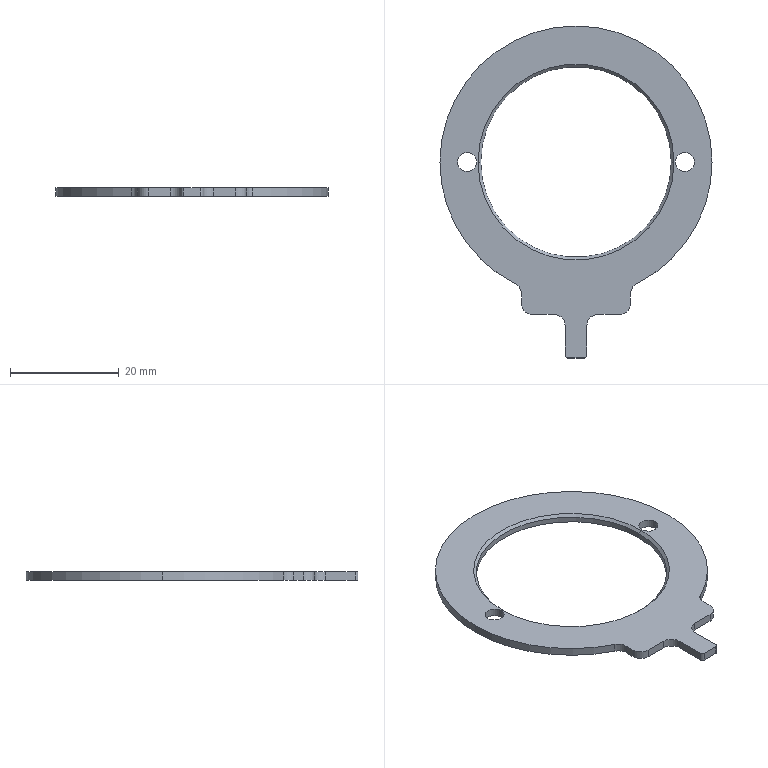Part | SolidWorks | features ICE 3, Fillet 2, Chamfer 1, Extrusion 1 | 1 solid | 28 faces | box 50 x 61 x 1.5 mm | volume 1619 mm3 | cylinder 17 | plane 9 | cone 2 | commonest cylinder face diameters 4 x6 3.5 x4 50 x3 1 x2 35 x2
STEP:
#1=CARTESIAN_POINT('',(-17.5,0.,1.));
#2=VERTEX_POINT('',#1);
#3=CARTESIAN_POINT('',(17.5,0.,1.));
#4=VERTEX_POINT('',#3);
#5=CARTESIAN_POINT('',(0.,0.,1.));
#6=DIRECTION('',(0.,0.,1.));
#7=DIRECTION('',(1.,0.,0.));
#8=AXIS2_PLACEMENT_3D('',#5,#6,#7);
#9=CIRCLE('',#8,17.5);
#10=EDGE_CURVE('',#2,#4,#9,.T.);
#11=ORIENTED_EDGE('',*,*,#10,.F.);
#12=CARTESIAN_POINT('',(-18.,0.,1.5));
#13=VERTEX_POINT('',#12);
#14=CARTESIAN_POINT('',(-17.5,0.,1.));
#15=DIRECTION('',(-0.7071,0.,0.7071));
#16=VECTOR('',#15,1000.);
#17=LINE('',#14,#16);
#18=EDGE_CURVE('',#2,#13,#17,.T.);
#19=ORIENTED_EDGE('',*,*,#18,.T.);
#20=CARTESIAN_POINT('',(18.,0.,1.5));
#21=VERTEX_POINT('',#20);
#22=CARTESIAN_POINT('',(0.,0.,1.5));
#23=DIRECTION('',(0.,0.,-1.));
#24=DIRECTION('',(1.,0.,0.));
#25=AXIS2_PLACEMENT_3D('',#22,#23,#24);
#26=CIRCLE('',#25,18.);
#27=EDGE_CURVE('',#21,#13,#26,.T.);
#28=ORIENTED_EDGE('',*,*,#27,.F.);
#29=CARTESIAN_POINT('',(17.5,0.,1.));
#30=DIRECTION('',(0.7071,0.,0.7071));
#31=VECTOR('',#30,1000.);
#32=LINE('',#29,#31);
#33=EDGE_CURVE('',#4,#21,#32,.T.);
#34=ORIENTED_EDGE('',*,*,#33,.F.);
#35=EDGE_LOOP('',(#11,#19,#28,#34));
#36=FACE_OUTER_BOUND('',#35,.T.);
#37=CARTESIAN_POINT('',(0.,0.,1.));
#38=DIRECTION('',(0.,0.,1.));
#39=DIRECTION('',(1.,0.,0.));
#40=AXIS2_PLACEMENT_3D('',#37,#38,#39);
#41=CONICAL_SURFACE('',#40,17.5,0.7854);
#42=ADVANCED_FACE('',(#36),#41,.F.);
#43=CARTESIAN_POINT('',(18.25,0.,0.));
#44=VERTEX_POINT('',#43);
#45=CARTESIAN_POINT('',(21.75,0.,0.));
#46=VERTEX_POINT('',#45);
#47=CARTESIAN_POINT('',(20.,0.,0.));
#48=DIRECTION('',(0.,0.,1.));
#49=DIRECTION('',(1.,0.,0.));
#50=AXIS2_PLACEMENT_3D('',#47,#48,#49);
#51=CIRCLE('',#50,1.75);
#52=EDGE_CURVE('',#44,#46,#51,.T.);
#53=ORIENTED_EDGE('',*,*,#52,.F.);
#54=CARTESIAN_POINT('',(18.25,0.,1.5));
#55=VERTEX_POINT('',#54);
#56=CARTESIAN_POINT('',(18.25,0.,-38.5));
#57=DIRECTION('',(0.,0.,1.));
#58=VECTOR('',#57,1000.);
#59=LINE('',#56,#58);
#60=EDGE_CURVE('',#44,#55,#59,.T.);
#61=ORIENTED_EDGE('',*,*,#60,.T.);
#62=CARTESIAN_POINT('',(21.75,0.,1.5));
#63=VERTEX_POINT('',#62);
#64=CARTESIAN_POINT('',(20.,0.,1.5));
#65=DIRECTION('',(0.,0.,1.));
#66=DIRECTION('',(1.,0.,0.));
#67=AXIS2_PLACEMENT_3D('',#64,#65,#66);
#68=CIRCLE('',#67,1.75);
#69=EDGE_CURVE('',#55,#63,#68,.T.);
#70=ORIENTED_EDGE('',*,*,#69,.T.);
#71=CARTESIAN_POINT('',(21.75,0.,-38.5));
#72=DIRECTION('',(0.,0.,1.));
#73=VECTOR('',#72,1000.);
#74=LINE('',#71,#73);
#75=EDGE_CURVE('',#46,#63,#74,.T.);
#76=ORIENTED_EDGE('',*,*,#75,.F.);
#77=EDGE_LOOP('',(#53,#61,#70,#76));
#78=FACE_OUTER_BOUND('',#77,.T.);
#79=CARTESIAN_POINT('',(20.,0.,-38.5));
#80=DIRECTION('',(0.,0.,1.));
#81=DIRECTION('',(1.,0.,0.));
#82=AXIS2_PLACEMENT_3D('',#79,#80,#81);
#83=CYLINDRICAL_SURFACE('',#82,1.75);
#84=ADVANCED_FACE('',(#78),#83,.F.);
#85=CARTESIAN_POINT('',(-21.75,0.,0.));
#86=VERTEX_POINT('',#85);
#87=CARTESIAN_POINT('',(-18.25,0.,0.));
#88=VERTEX_POINT('',#87);
#89=CARTESIAN_POINT('',(-20.,0.,0.));
#90=DIRECTION('',(0.,0.,1.));
#91=DIRECTION('',(1.,0.,0.));
#92=AXIS2_PLACEMENT_3D('',#89,#90,#91);
#93=CIRCLE('',#92,1.75);
#94=EDGE_CURVE('',#86,#88,#93,.T.);
#95=ORIENTED_EDGE('',*,*,#94,.F.);
#96=CARTESIAN_POINT('',(-21.75,0.,1.5));
#97=VERTEX_POINT('',#96);
#98=CARTESIAN_POINT('',(-21.75,0.,-38.5));
#99=DIRECTION('',(0.,0.,1.));
#100=VECTOR('',#99,1000.);
#101=LINE('',#98,#100);
#102=EDGE_CURVE('',#86,#97,#101,.T.);
#103=ORIENTED_EDGE('',*,*,#102,.T.);
#104=CARTESIAN_POINT('',(-18.25,0.,1.5));
#105=VERTEX_POINT('',#104);
#106=CARTESIAN_POINT('',(-20.,0.,1.5));
#107=DIRECTION('',(0.,0.,1.));
#108=DIRECTION('',(1.,0.,0.));
#109=AXIS2_PLACEMENT_3D('',#106,#107,#108);
#110=CIRCLE('',#109,1.75);
#111=EDGE_CURVE('',#97,#105,#110,.T.);
#112=ORIENTED_EDGE('',*,*,#111,.T.);
#113=CARTESIAN_POINT('',(-18.25,0.,-38.5));
#114=DIRECTION('',(0.,0.,1.));
#115=VECTOR('',#114,1000.);
#116=LINE('',#113,#115);
#117=EDGE_CURVE('',#88,#105,#116,.T.);
#118=ORIENTED_EDGE('',*,*,#117,.F.);
#119=EDGE_LOOP('',(#95,#103,#112,#118));
#120=FACE_OUTER_BOUND('',#119,.T.);
#121=CARTESIAN_POINT('',(-20.,0.,-38.5));
#122=DIRECTION('',(0.,0.,1.));
#123=DIRECTION('',(1.,0.,0.));
#124=AXIS2_PLACEMENT_3D('',#121,#122,#123);
#125=CYLINDRICAL_SURFACE('',#124,1.75);
#126=ADVANCED_FACE('',(#120),#125,.F.);
#127=ORIENTED_EDGE('',*,*,#10,.T.);
#128=CARTESIAN_POINT('',(17.5,0.,0.));
#129=VERTEX_POINT('',#128);
#130=CARTESIAN_POINT('',(17.5,0.,1.5));
#131=DIRECTION('',(0.,0.,-1.));
#132=VECTOR('',#131,1000.);
#133=LINE('',#130,#132);
#134=EDGE_CURVE('',#4,#129,#133,.T.);
#135=ORIENTED_EDGE('',*,*,#134,.T.);
#136=CARTESIAN_POINT('',(-17.5,0.,0.));
#137=VERTEX_POINT('',#136);
#138=CARTESIAN_POINT('',(0.,0.,0.));
#139=DIRECTION('',(0.,0.,1.));
#140=DIRECTION('',(1.,0.,0.));
#141=AXIS2_PLACEMENT_3D('',#138,#139,#140);
#142=CIRCLE('',#141,17.5);
#143=EDGE_CURVE('',#137,#129,#142,.T.);
#144=ORIENTED_EDGE('',*,*,#143,.F.);
#145=CARTESIAN_POINT('',(-17.5,0.,1.5));
#146=DIRECTION('',(0.,0.,-1.));
#147=VECTOR('',#146,1000.);
#148=LINE('',#145,#147);
#149=EDGE_CURVE('',#2,#137,#148,.T.);
#150=ORIENTED_EDGE('',*,*,#149,.F.);
#151=EDGE_LOOP('',(#127,#135,#144,#150));
#152=FACE_OUTER_BOUND('',#151,.T.);
#153=CARTESIAN_POINT('',(0.,0.,1.5));
#154=DIRECTION('',(0.,0.,-1.));
#155=DIRECTION('',(-1.,0.,0.));
#156=AXIS2_PLACEMENT_3D('',#153,#154,#155);
#157=CYLINDRICAL_SURFACE('',#156,17.5);
#158=ADVANCED_FACE('',(#152),#157,.F.);
#159=CARTESIAN_POINT('',(25.,0.,1.5));
#160=VERTEX_POINT('',#159);
#161=CARTESIAN_POINT('',(-25.,0.,1.5));
#162=VERTEX_POINT('',#161);
#163=CARTESIAN_POINT('',(0.,0.,1.5));
#164=DIRECTION('',(0.,0.,1.));
#165=DIRECTION('',(1.,0.,0.));
#166=AXIS2_PLACEMENT_3D('',#163,#164,#165);
#167=CIRCLE('',#166,25.);
#168=EDGE_CURVE('',#160,#162,#167,.T.);
#169=ORIENTED_EDGE('',*,*,#168,.F.);
#170=CARTESIAN_POINT('',(25.,0.,0.));
#171=VERTEX_POINT('',#170);
#172=CARTESIAN_POINT('',(25.,0.,1.5));
#173=DIRECTION('',(0.,0.,-1.));
#174=VECTOR('',#173,1000.);
#175=LINE('',#172,#174);
#176=EDGE_CURVE('',#160,#171,#175,.T.);
#177=ORIENTED_EDGE('',*,*,#176,.T.);
#178=CARTESIAN_POINT('',(-25.,0.,0.));
#179=VERTEX_POINT('',#178);
#180=CARTESIAN_POINT('',(0.,0.,0.));
#181=DIRECTION('',(0.,0.,1.));
#182=DIRECTION('',(1.,0.,0.));
#183=AXIS2_PLACEMENT_3D('',#180,#181,#182);
#184=CIRCLE('',#183,25.);
#185=EDGE_CURVE('',#171,#179,#184,.T.);
#186=ORIENTED_EDGE('',*,*,#185,.T.);
#187=CARTESIAN_POINT('',(-25.,0.,1.5));
#188=DIRECTION('',(0.,0.,-1.));
#189=VECTOR('',#188,1000.);
#190=LINE('',#187,#189);
#191=EDGE_CURVE('',#162,#179,#190,.T.);
#192=ORIENTED_EDGE('',*,*,#191,.F.);
#193=EDGE_LOOP('',(#169,#177,#186,#192));
#194=FACE_OUTER_BOUND('',#193,.T.);
#195=CARTESIAN_POINT('',(0.,0.,1.5));
#196=DIRECTION('',(0.,0.,-1.));
#197=DIRECTION('',(-1.,0.,0.));
#198=AXIS2_PLACEMENT_3D('',#195,#196,#197);
#199=CYLINDRICAL_SURFACE('',#198,25.);
#200=ADVANCED_FACE('',(#194),#199,.T.);
#201=CARTESIAN_POINT('',(-11.111,-22.395,1.5));
#202=VERTEX_POINT('',#201);
#203=CARTESIAN_POINT('',(0.,0.,1.5));
#204=DIRECTION('',(0.,0.,1.));
#205=DIRECTION('',(1.,0.,0.));
#206=AXIS2_PLACEMENT_3D('',#203,#204,#205);
#207=CIRCLE('',#206,25.);
#208=EDGE_CURVE('',#162,#202,#207,.T.);
#209=ORIENTED_EDGE('',*,*,#208,.F.);
#210=ORIENTED_EDGE('',*,*,#191,.T.);
#211=CARTESIAN_POINT('',(-11.111,-22.395,0.));
#212=VERTEX_POINT('',#211);
#213=CARTESIAN_POINT('',(0.,0.,0.));
#214=DIRECTION('',(0.,0.,1.));
#215=DIRECTION('',(1.,0.,0.));
#216=AXIS2_PLACEMENT_3D('',#213,#214,#215);
#217=CIRCLE('',#216,25.);
#218=EDGE_CURVE('',#179,#212,#217,.T.);
#219=ORIENTED_EDGE('',*,*,#218,.T.);
#220=CARTESIAN_POINT('',(-11.111,-22.395,1.5));
#221=DIRECTION('',(0.,0.,1.));
#222=VECTOR('',#221,1000.);
#223=LINE('',#220,#222);
#224=EDGE_CURVE('',#212,#202,#223,.T.);
#225=ORIENTED_EDGE('',*,*,#224,.T.);
#226=EDGE_LOOP('',(#209,#210,#219,#225));
#227=FACE_OUTER_BOUND('',#226,.T.);
#228=CARTESIAN_POINT('',(0.,0.,1.5));
#229=DIRECTION('',(0.,0.,-1.));
#230=DIRECTION('',(-1.,0.,0.));
#231=AXIS2_PLACEMENT_3D('',#228,#229,#230);
#232=CYLINDRICAL_SURFACE('',#231,25.);
#233=ADVANCED_FACE('',(#227),#232,.T.);
#234=ORIENTED_EDGE('',*,*,#27,.T.);
#235=CARTESIAN_POINT('',(0.,0.,1.5));
#236=DIRECTION('',(0.,0.,-1.));
#237=DIRECTION('',(1.,0.,0.));
#238=AXIS2_PLACEMENT_3D('',#235,#236,#237);
#239=CIRCLE('',#238,18.);
#240=EDGE_CURVE('',#13,#21,#239,.T.);
#241=ORIENTED_EDGE('',*,*,#240,.T.);
#242=EDGE_LOOP('',(#234,#241));
#243=FACE_BOUND('',#242,.T.);
#244=CARTESIAN_POINT('',(20.,0.,1.5));
#245=DIRECTION('',(0.,0.,1.));
#246=DIRECTION('',(1.,0.,0.));
#247=AXIS2_PLACEMENT_3D('',#244,#245,#246);
#248=CIRCLE('',#247,1.75);
#249=EDGE_CURVE('',#63,#55,#248,.T.);
#250=ORIENTED_EDGE('',*,*,#249,.F.);
#251=ORIENTED_EDGE('',*,*,#69,.F.);
#252=EDGE_LOOP('',(#250,#251));
#253=FACE_BOUND('',#252,.T.);
#254=CARTESIAN_POINT('',(-20.,0.,1.5));
#255=DIRECTION('',(0.,0.,1.));
#256=DIRECTION('',(1.,0.,0.));
#257=AXIS2_PLACEMENT_3D('',#254,#255,#256);
#258=CIRCLE('',#257,1.75);
#259=EDGE_CURVE('',#105,#97,#258,.T.);
#260=ORIENTED_EDGE('',*,*,#259,.F.);
#261=ORIENTED_EDGE('',*,*,#111,.F.);
#262=EDGE_LOOP('',(#260,#261));
#263=FACE_BOUND('',#262,.T.);
#264=CARTESIAN_POINT('',(-1.5,-36.,1.5));
#265=VERTEX_POINT('',#264);
#266=CARTESIAN_POINT('',(1.5,-36.,1.5));
#267=VERTEX_POINT('',#266);
#268=CARTESIAN_POINT('',(-10.,-36.,1.5));
#269=DIRECTION('',(1.,0.,0.));
#270=VECTOR('',#269,1000.);
#271=LINE('',#268,#270);
#272=EDGE_CURVE('',#265,#267,#271,.T.);
#273=ORIENTED_EDGE('',*,*,#272,.T.);
#274=CARTESIAN_POINT('',(2.,-35.5,1.5));
#275=VERTEX_POINT('',#274);
#276=CARTESIAN_POINT('',(1.5,-35.5,1.5));
#277=DIRECTION('',(0.,0.,1.));
#278=DIRECTION('',(1.,0.,0.));
#279=AXIS2_PLACEMENT_3D('',#276,#277,#278);
#280=CIRCLE('',#279,0.5);
#281=EDGE_CURVE('',#267,#275,#280,.T.);
#282=ORIENTED_EDGE('',*,*,#281,.T.);
#283=CARTESIAN_POINT('',(2.,-30.,1.5));
#284=VERTEX_POINT('',#283);
#285=CARTESIAN_POINT('',(2.,-36.,1.5));
#286=DIRECTION('',(0.,-1.,0.));
#287=VECTOR('',#286,1000.);
#288=LINE('',#285,#287);
#289=EDGE_CURVE('',#284,#275,#288,.T.);
#290=ORIENTED_EDGE('',*,*,#289,.F.);
#291=CARTESIAN_POINT('',(4.,-28.,1.5));
#292=VERTEX_POINT('',#291);
#293=CARTESIAN_POINT('',(4.,-30.,1.5));
#294=DIRECTION('',(0.,0.,-1.));
#295=DIRECTION('',(1.,0.,0.));
#296=AXIS2_PLACEMENT_3D('',#293,#294,#295);
#297=CIRCLE('',#296,2.);
#298=EDGE_CURVE('',#284,#292,#297,.T.);
#299=ORIENTED_EDGE('',*,*,#298,.T.);
#300=CARTESIAN_POINT('',(8.,-28.,1.5));
#301=VERTEX_POINT('',#300);
#302=CARTESIAN_POINT('',(10.,-28.,1.5));
#303=DIRECTION('',(-1.,0.,0.));
#304=VECTOR('',#303,1000.);
#305=LINE('',#302,#304);
#306=EDGE_CURVE('',#301,#292,#305,.T.);
#307=ORIENTED_EDGE('',*,*,#306,.F.);
#308=CARTESIAN_POINT('',(10.,-26.,1.5));
#309=VERTEX_POINT('',#308);
#310=CARTESIAN_POINT('',(8.,-26.,1.5));
#311=DIRECTION('',(0.,0.,1.));
#312=DIRECTION('',(1.,0.,0.));
#313=AXIS2_PLACEMENT_3D('',#310,#311,#312);
#314=CIRCLE('',#313,2.);
#315=EDGE_CURVE('',#301,#309,#314,.T.);
#316=ORIENTED_EDGE('',*,*,#315,.T.);
#317=CARTESIAN_POINT('',(10.,-24.187,1.5));
#318=VERTEX_POINT('',#317);
#319=CARTESIAN_POINT('',(10.,-21.,1.5));
#320=DIRECTION('',(0.,1.,0.));
#321=VECTOR('',#320,1000.);
#322=LINE('',#319,#321);
#323=EDGE_CURVE('',#309,#318,#322,.T.);
#324=ORIENTED_EDGE('',*,*,#323,.T.);
#325=CARTESIAN_POINT('',(11.111,-22.395,1.5));
#326=VERTEX_POINT('',#325);
#327=CARTESIAN_POINT('',(12.,-24.187,1.5));
#328=DIRECTION('',(0.,0.,-1.));
#329=DIRECTION('',(1.,0.,0.));
#330=AXIS2_PLACEMENT_3D('',#327,#328,#329);
#331=CIRCLE('',#330,2.);
#332=EDGE_CURVE('',#318,#326,#331,.T.);
#333=ORIENTED_EDGE('',*,*,#332,.T.);
#334=CARTESIAN_POINT('',(0.,0.,1.5));
#335=DIRECTION('',(0.,0.,1.));
#336=DIRECTION('',(1.,0.,0.));
#337=AXIS2_PLACEMENT_3D('',#334,#335,#336);
#338=CIRCLE('',#337,25.);
#339=EDGE_CURVE('',#326,#160,#338,.T.);
#340=ORIENTED_EDGE('',*,*,#339,.T.);
#341=ORIENTED_EDGE('',*,*,#168,.T.);
#342=ORIENTED_EDGE('',*,*,#208,.T.);
#343=CARTESIAN_POINT('',(-10.,-24.187,1.5));
#344=VERTEX_POINT('',#343);
#345=CARTESIAN_POINT('',(-12.,-24.187,1.5));
#346=DIRECTION('',(0.,0.,-1.));
#347=DIRECTION('',(1.,0.,0.));
#348=AXIS2_PLACEMENT_3D('',#345,#346,#347);
#349=CIRCLE('',#348,2.);
#350=EDGE_CURVE('',#202,#344,#349,.T.);
#351=ORIENTED_EDGE('',*,*,#350,.T.);
#352=CARTESIAN_POINT('',(-10.,-26.,1.5));
#353=VERTEX_POINT('',#352);
#354=CARTESIAN_POINT('',(-10.,-21.,1.5));
#355=DIRECTION('',(0.,-1.,0.));
#356=VECTOR('',#355,1000.);
#357=LINE('',#354,#356);
#358=EDGE_CURVE('',#344,#353,#357,.T.);
#359=ORIENTED_EDGE('',*,*,#358,.T.);
#360=CARTESIAN_POINT('',(-8.,-28.,1.5));
#361=VERTEX_POINT('',#360);
#362=CARTESIAN_POINT('',(-8.,-26.,1.5));
#363=DIRECTION('',(0.,0.,1.));
#364=DIRECTION('',(1.,0.,0.));
#365=AXIS2_PLACEMENT_3D('',#362,#363,#364);
#366=CIRCLE('',#365,2.);
#367=EDGE_CURVE('',#353,#361,#366,.T.);
#368=ORIENTED_EDGE('',*,*,#367,.T.);
#369=CARTESIAN_POINT('',(-4.,-28.,1.5));
#370=VERTEX_POINT('',#369);
#371=CARTESIAN_POINT('',(-10.,-28.,1.5));
#372=DIRECTION('',(-1.,0.,0.));
#373=VECTOR('',#372,1000.);
#374=LINE('',#371,#373);
#375=EDGE_CURVE('',#370,#361,#374,.T.);
#376=ORIENTED_EDGE('',*,*,#375,.F.);
#377=CARTESIAN_POINT('',(-2.,-30.,1.5));
#378=VERTEX_POINT('',#377);
#379=CARTESIAN_POINT('',(-4.,-30.,1.5));
#380=DIRECTION('',(0.,0.,-1.));
#381=DIRECTION('',(1.,0.,0.));
#382=AXIS2_PLACEMENT_3D('',#379,#380,#381);
#383=CIRCLE('',#382,2.);
#384=EDGE_CURVE('',#370,#378,#383,.T.);
#385=ORIENTED_EDGE('',*,*,#384,.T.);
#386=CARTESIAN_POINT('',(-2.,-35.5,1.5));
#387=VERTEX_POINT('',#386);
#388=CARTESIAN_POINT('',(-2.,-36.,1.5));
#389=DIRECTION('',(0.,1.,0.));
#390=VECTOR('',#389,1000.);
#391=LINE('',#388,#390);
#392=EDGE_CURVE('',#387,#378,#391,.T.);
#393=ORIENTED_EDGE('',*,*,#392,.F.);
#394=CARTESIAN_POINT('',(-1.5,-35.5,1.5));
#395=DIRECTION('',(0.,0.,1.));
#396=DIRECTION('',(1.,0.,0.));
#397=AXIS2_PLACEMENT_3D('',#394,#395,#396);
#398=CIRCLE('',#397,0.5);
#399=EDGE_CURVE('',#387,#265,#398,.T.);
#400=ORIENTED_EDGE('',*,*,#399,.T.);
#401=EDGE_LOOP('',(#273,#282,#290,#299,#307,#316,#324,#333,#340,#341,#342,#351,#359,#368,#376,#385,#393,#400));
#402=FACE_OUTER_BOUND('',#401,.T.);
#403=CARTESIAN_POINT('',(0.,0.,1.5));
#404=DIRECTION('',(0.,0.,1.));
#405=DIRECTION('',(1.,0.,0.));
#406=AXIS2_PLACEMENT_3D('',#403,#404,#405);
#407=PLANE('',#406);
#408=ADVANCED_FACE('',(#243,#253,#263,#402),#407,.T.);
#409=CARTESIAN_POINT('',(20.,0.,0.));
#410=DIRECTION('',(0.,0.,1.));
#411=DIRECTION('',(1.,0.,0.));
#412=AXIS2_PLACEMENT_3D('',#409,#410,#411);
#413=CIRCLE('',#412,1.75);
#414=EDGE_CURVE('',#46,#44,#413,.T.);
#415=ORIENTED_EDGE('',*,*,#414,.T.);
#416=ORIENTED_EDGE('',*,*,#52,.T.);
#417=EDGE_LOOP('',(#415,#416));
#418=FACE_BOUND('',#417,.T.);
#419=CARTESIAN_POINT('',(-20.,0.,0.));
#420=DIRECTION('',(0.,0.,1.));
#421=DIRECTION('',(1.,0.,0.));
#422=AXIS2_PLACEMENT_3D('',#419,#420,#421);
#423=CIRCLE('',#422,1.75);
#424=EDGE_CURVE('',#88,#86,#423,.T.);
#425=ORIENTED_EDGE('',*,*,#424,.T.);
#426=ORIENTED_EDGE('',*,*,#94,.T.);
#427=EDGE_LOOP('',(#425,#426));
#428=FACE_BOUND('',#427,.T.);
#429=CARTESIAN_POINT('',(2.,-30.,0.));
#430=VERTEX_POINT('',#429);
#431=CARTESIAN_POINT('',(2.,-35.5,0.));
#432=VERTEX_POINT('',#431);
#433=CARTESIAN_POINT('',(2.,0.,0.));
#434=DIRECTION('',(0.,-1.,0.));
#435=VECTOR('',#434,1000.);
#436=LINE('',#433,#435);
#437=EDGE_CURVE('',#430,#432,#436,.T.);
#438=ORIENTED_EDGE('',*,*,#437,.T.);
#439=CARTESIAN_POINT('',(1.5,-36.,0.));
#440=VERTEX_POINT('',#439);
#441=CARTESIAN_POINT('',(1.5,-35.5,0.));
#442=DIRECTION('',(0.,0.,-1.));
#443=DIRECTION('',(1.,0.,0.));
#444=AXIS2_PLACEMENT_3D('',#441,#442,#443);
#445=CIRCLE('',#444,0.5);
#446=EDGE_CURVE('',#432,#440,#445,.T.);
#447=ORIENTED_EDGE('',*,*,#446,.T.);
#448=CARTESIAN_POINT('',(-1.5,-36.,0.));
#449=VERTEX_POINT('',#448);
#450=CARTESIAN_POINT('',(-10.,-36.,0.));
#451=DIRECTION('',(-1.,0.,0.));
#452=VECTOR('',#451,1000.);
#453=LINE('',#450,#452);
#454=EDGE_CURVE('',#440,#449,#453,.T.);
#455=ORIENTED_EDGE('',*,*,#454,.T.);
#456=CARTESIAN_POINT('',(-2.,-35.5,0.));
#457=VERTEX_POINT('',#456);
#458=CARTESIAN_POINT('',(-1.5,-35.5,0.));
#459=DIRECTION('',(0.,0.,-1.));
#460=DIRECTION('',(1.,0.,0.));
#461=AXIS2_PLACEMENT_3D('',#458,#459,#460);
#462=CIRCLE('',#461,0.5);
#463=EDGE_CURVE('',#449,#457,#462,.T.);
#464=ORIENTED_EDGE('',*,*,#463,.T.);
#465=CARTESIAN_POINT('',(-2.,-30.,0.));
#466=VERTEX_POINT('',#465);
#467=CARTESIAN_POINT('',(-2.,0.,0.));
#468=DIRECTION('',(0.,1.,0.));
#469=VECTOR('',#468,1000.);
#470=LINE('',#467,#469);
#471=EDGE_CURVE('',#457,#466,#470,.T.);
#472=ORIENTED_EDGE('',*,*,#471,.T.);
#473=CARTESIAN_POINT('',(-4.,-28.,0.));
#474=VERTEX_POINT('',#473);
#475=CARTESIAN_POINT('',(-4.,-30.,0.));
#476=DIRECTION('',(0.,0.,1.));
#477=DIRECTION('',(1.,0.,0.));
#478=AXIS2_PLACEMENT_3D('',#475,#476,#477);
#479=CIRCLE('',#478,2.);
#480=EDGE_CURVE('',#466,#474,#479,.T.);
#481=ORIENTED_EDGE('',*,*,#480,.T.);
#482=CARTESIAN_POINT('',(-8.,-28.,0.));
#483=VERTEX_POINT('',#482);
#484=CARTESIAN_POINT('',(0.,-28.,0.));
#485=DIRECTION('',(-1.,0.,0.));
#486=VECTOR('',#485,1000.);
#487=LINE('',#484,#486);
#488=EDGE_CURVE('',#474,#483,#487,.T.);
#489=ORIENTED_EDGE('',*,*,#488,.T.);
#490=CARTESIAN_POINT('',(-10.,-26.,0.));
#491=VERTEX_POINT('',#490);
#492=CARTESIAN_POINT('',(-8.,-26.,0.));
#493=DIRECTION('',(0.,0.,-1.));
#494=DIRECTION('',(1.,0.,0.));
#495=AXIS2_PLACEMENT_3D('',#492,#493,#494);
#496=CIRCLE('',#495,2.);
#497=EDGE_CURVE('',#483,#491,#496,.T.);
#498=ORIENTED_EDGE('',*,*,#497,.T.);
#499=CARTESIAN_POINT('',(-10.,-24.187,0.));
#500=VERTEX_POINT('',#499);
#501=CARTESIAN_POINT('',(-10.,-21.,0.));
#502=DIRECTION('',(0.,1.,0.));
#503=VECTOR('',#502,1000.);
#504=LINE('',#501,#503);
#505=EDGE_CURVE('',#491,#500,#504,.T.);
#506=ORIENTED_EDGE('',*,*,#505,.T.);
#507=CARTESIAN_POINT('',(-12.,-24.187,0.));
#508=DIRECTION('',(0.,0.,1.));
#509=DIRECTION('',(1.,0.,0.));
#510=AXIS2_PLACEMENT_3D('',#507,#508,#509);
#511=CIRCLE('',#510,2.);
#512=EDGE_CURVE('',#500,#212,#511,.T.);
#513=ORIENTED_EDGE('',*,*,#512,.T.);
#514=ORIENTED_EDGE('',*,*,#218,.F.);
#515=ORIENTED_EDGE('',*,*,#185,.F.);
#516=CARTESIAN_POINT('',(11.111,-22.395,0.));
#517=VERTEX_POINT('',#516);
#518=CARTESIAN_POINT('',(0.,0.,0.));
#519=DIRECTION('',(0.,0.,1.));
#520=DIRECTION('',(1.,0.,0.));
#521=AXIS2_PLACEMENT_3D('',#518,#519,#520);
#522=CIRCLE('',#521,25.);
#523=EDGE_CURVE('',#517,#171,#522,.T.);
#524=ORIENTED_EDGE('',*,*,#523,.F.);
#525=CARTESIAN_POINT('',(10.,-24.187,0.));
#526=VERTEX_POINT('',#525);
#527=CARTESIAN_POINT('',(12.,-24.187,0.));
#528=DIRECTION('',(0.,0.,1.));
#529=DIRECTION('',(1.,0.,0.));
#530=AXIS2_PLACEMENT_3D('',#527,#528,#529);
#531=CIRCLE('',#530,2.);
#532=EDGE_CURVE('',#517,#526,#531,.T.);
#533=ORIENTED_EDGE('',*,*,#532,.T.);
#534=CARTESIAN_POINT('',(10.,-26.,0.));
#535=VERTEX_POINT('',#534);
#536=CARTESIAN_POINT('',(10.,-21.,0.));
#537=DIRECTION('',(0.,-1.,0.));
#538=VECTOR('',#537,1000.);
#539=LINE('',#536,#538);
#540=EDGE_CURVE('',#526,#535,#539,.T.);
#541=ORIENTED_EDGE('',*,*,#540,.T.);
#542=CARTESIAN_POINT('',(8.,-28.,0.));
#543=VERTEX_POINT('',#542);
#544=CARTESIAN_POINT('',(8.,-26.,0.));
#545=DIRECTION('',(0.,0.,-1.));
#546=DIRECTION('',(1.,0.,0.));
#547=AXIS2_PLACEMENT_3D('',#544,#545,#546);
#548=CIRCLE('',#547,2.);
#549=EDGE_CURVE('',#535,#543,#548,.T.);
#550=ORIENTED_EDGE('',*,*,#549,.T.);
#551=CARTESIAN_POINT('',(4.,-28.,0.));
#552=VERTEX_POINT('',#551);
#553=CARTESIAN_POINT('',(0.,-28.,0.));
#554=DIRECTION('',(-1.,0.,0.));
#555=VECTOR('',#554,1000.);
#556=LINE('',#553,#555);
#557=EDGE_CURVE('',#543,#552,#556,.T.);
#558=ORIENTED_EDGE('',*,*,#557,.T.);
#559=CARTESIAN_POINT('',(4.,-30.,0.));
#560=DIRECTION('',(0.,0.,1.));
#561=DIRECTION('',(1.,0.,0.));
#562=AXIS2_PLACEMENT_3D('',#559,#560,#561);
#563=CIRCLE('',#562,2.);
#564=EDGE_CURVE('',#552,#430,#563,.T.);
#565=ORIENTED_EDGE('',*,*,#564,.T.);
#566=EDGE_LOOP('',(#438,#447,#455,#464,#472,#481,#489,#498,#506,#513,#514,#515,#524,#533,#541,#550,#558,#565));
#567=FACE_OUTER_BOUND('',#566,.T.);
#568=ORIENTED_EDGE('',*,*,#143,.T.);
#569=CARTESIAN_POINT('',(0.,0.,0.));
#570=DIRECTION('',(0.,0.,1.));
#571=DIRECTION('',(1.,0.,0.));
#572=AXIS2_PLACEMENT_3D('',#569,#570,#571);
#573=CIRCLE('',#572,17.5);
#574=EDGE_CURVE('',#129,#137,#573,.T.);
#575=ORIENTED_EDGE('',*,*,#574,.T.);
#576=EDGE_LOOP('',(#568,#575));
#577=FACE_BOUND('',#576,.T.);
#578=CARTESIAN_POINT('',(0.,0.,0.));
#579=DIRECTION('',(0.,0.,1.));
#580=DIRECTION('',(1.,0.,0.));
#581=AXIS2_PLACEMENT_3D('',#578,#579,#580);
#582=PLANE('',#581);
#583=ADVANCED_FACE('',(#418,#428,#567,#577),#582,.F.);
#584=ORIENTED_EDGE('',*,*,#176,.F.);
#585=ORIENTED_EDGE('',*,*,#339,.F.);
#586=CARTESIAN_POINT('',(11.111,-22.395,1.5));
#587=DIRECTION('',(0.,0.,-1.));
#588=VECTOR('',#587,1000.);
#589=LINE('',#586,#588);
#590=EDGE_CURVE('',#326,#517,#589,.T.);
#591=ORIENTED_EDGE('',*,*,#590,.T.);
#592=ORIENTED_EDGE('',*,*,#523,.T.);
#593=EDGE_LOOP('',(#584,#585,#591,#592));
#594=FACE_OUTER_BOUND('',#593,.T.);
#595=CARTESIAN_POINT('',(0.,0.,1.5));
#596=DIRECTION('',(0.,0.,-1.));
#597=DIRECTION('',(-1.,0.,0.));
#598=AXIS2_PLACEMENT_3D('',#595,#596,#597);
#599=CYLINDRICAL_SURFACE('',#598,25.);
#600=ADVANCED_FACE('',(#594),#599,.T.);
#601=ORIENTED_EDGE('',*,*,#134,.F.);
#602=CARTESIAN_POINT('',(0.,0.,1.));
#603=DIRECTION('',(0.,0.,1.));
#604=DIRECTION('',(1.,0.,0.));
#605=AXIS2_PLACEMENT_3D('',#602,#603,#604);
#606=CIRCLE('',#605,17.5);
#607=EDGE_CURVE('',#4,#2,#606,.T.);
#608=ORIENTED_EDGE('',*,*,#607,.T.);
#609=ORIENTED_EDGE('',*,*,#149,.T.);
#610=ORIENTED_EDGE('',*,*,#574,.F.);
#611=EDGE_LOOP('',(#601,#608,#609,#610));
#612=FACE_OUTER_BOUND('',#611,.T.);
#613=CARTESIAN_POINT('',(0.,0.,1.5));
#614=DIRECTION('',(0.,0.,-1.));
#615=DIRECTION('',(-1.,0.,0.));
#616=AXIS2_PLACEMENT_3D('',#613,#614,#615);
#617=CYLINDRICAL_SURFACE('',#616,17.5);
#618=ADVANCED_FACE('',(#612),#617,.F.);
#619=ORIENTED_EDGE('',*,*,#505,.F.);
#620=CARTESIAN_POINT('',(-10.,-26.,1.5));
#621=DIRECTION('',(0.,0.,1.));
#622=VECTOR('',#621,1000.);
#623=LINE('',#620,#622);
#624=EDGE_CURVE('',#491,#353,#623,.T.);
#625=ORIENTED_EDGE('',*,*,#624,.T.);
#626=ORIENTED_EDGE('',*,*,#358,.F.);
#627=CARTESIAN_POINT('',(-10.,-24.187,-25.));
#628=DIRECTION('',(0.,0.,-1.));
#629=VECTOR('',#628,1000.);
#630=LINE('',#627,#629);
#631=EDGE_CURVE('',#344,#500,#630,.T.);
#632=ORIENTED_EDGE('',*,*,#631,.T.);
#633=EDGE_LOOP('',(#619,#625,#626,#632));
#634=FACE_OUTER_BOUND('',#633,.T.);
#635=CARTESIAN_POINT('',(-10.,-21.,-25.));
#636=DIRECTION('',(-1.,0.,0.));
#637=DIRECTION('',(0.,-1.,0.));
#638=AXIS2_PLACEMENT_3D('',#635,#636,#637);
#639=PLANE('',#638);
#640=ADVANCED_FACE('',(#634),#639,.T.);
#641=ORIENTED_EDGE('',*,*,#323,.F.);
#642=CARTESIAN_POINT('',(10.,-26.,0.));
#643=DIRECTION('',(0.,0.,-1.));
#644=VECTOR('',#643,1000.);
#645=LINE('',#642,#644);
#646=EDGE_CURVE('',#309,#535,#645,.T.);
#647=ORIENTED_EDGE('',*,*,#646,.T.);
#648=ORIENTED_EDGE('',*,*,#540,.F.);
#649=CARTESIAN_POINT('',(10.,-24.187,-25.));
#650=DIRECTION('',(0.,0.,1.));
#651=VECTOR('',#650,1000.);
#652=LINE('',#649,#651);
#653=EDGE_CURVE('',#526,#318,#652,.T.);
#654=ORIENTED_EDGE('',*,*,#653,.T.);
#655=EDGE_LOOP('',(#641,#647,#648,#654));
#656=FACE_OUTER_BOUND('',#655,.T.);
#657=CARTESIAN_POINT('',(10.,-21.,-25.));
#658=DIRECTION('',(1.,0.,0.));
#659=DIRECTION('',(0.,1.,0.));
#660=AXIS2_PLACEMENT_3D('',#657,#658,#659);
#661=PLANE('',#660);
#662=ADVANCED_FACE('',(#656),#661,.T.);
#663=ORIENTED_EDGE('',*,*,#454,.F.);
#664=CARTESIAN_POINT('',(1.5,-36.,1.5));
#665=DIRECTION('',(0.,0.,1.));
#666=VECTOR('',#665,1000.);
#667=LINE('',#664,#666);
#668=EDGE_CURVE('',#440,#267,#667,.T.);
#669=ORIENTED_EDGE('',*,*,#668,.T.);
#670=ORIENTED_EDGE('',*,*,#272,.F.);
#671=CARTESIAN_POINT('',(-1.5,-36.,0.));
#672=DIRECTION('',(0.,0.,-1.));
#673=VECTOR('',#672,1000.);
#674=LINE('',#671,#673);
#675=EDGE_CURVE('',#265,#449,#674,.T.);
#676=ORIENTED_EDGE('',*,*,#675,.T.);
#677=EDGE_LOOP('',(#663,#669,#670,#676));
#678=FACE_OUTER_BOUND('',#677,.T.);
#679=CARTESIAN_POINT('',(-10.,-36.,-25.));
#680=DIRECTION('',(0.,-1.,0.));
#681=DIRECTION('',(0.,0.,-1.));
#682=AXIS2_PLACEMENT_3D('',#679,#680,#681);
#683=PLANE('',#682);
#684=ADVANCED_FACE('',(#678),#683,.T.);
#685=ORIENTED_EDGE('',*,*,#375,.T.);
#686=CARTESIAN_POINT('',(-8.,-28.,0.));
#687=DIRECTION('',(0.,0.,-1.));
#688=VECTOR('',#687,1000.);
#689=LINE('',#686,#688);
#690=EDGE_CURVE('',#361,#483,#689,.T.);
#691=ORIENTED_EDGE('',*,*,#690,.T.);
#692=ORIENTED_EDGE('',*,*,#488,.F.);
#693=CARTESIAN_POINT('',(-4.,-28.,1.5));
#694=DIRECTION('',(0.,0.,1.));
#695=VECTOR('',#694,1000.);
#696=LINE('',#693,#695);
#697=EDGE_CURVE('',#474,#370,#696,.T.);
#698=ORIENTED_EDGE('',*,*,#697,.T.);
#699=EDGE_LOOP('',(#685,#691,#692,#698));
#700=FACE_OUTER_BOUND('',#699,.T.);
#701=CARTESIAN_POINT('',(-10.,-28.,-18.5));
#702=DIRECTION('',(0.,1.,0.));
#703=DIRECTION('',(0.,0.,1.));
#704=AXIS2_PLACEMENT_3D('',#701,#702,#703);
#705=PLANE('',#704);
#706=ADVANCED_FACE('',(#700),#705,.F.);
#707=ORIENTED_EDGE('',*,*,#471,.F.);
#708=CARTESIAN_POINT('',(-2.,-35.5,1.5));
#709=DIRECTION('',(0.,0.,1.));
#710=VECTOR('',#709,1000.);
#711=LINE('',#708,#710);
#712=EDGE_CURVE('',#457,#387,#711,.T.);
#713=ORIENTED_EDGE('',*,*,#712,.T.);
#714=ORIENTED_EDGE('',*,*,#392,.T.);
#715=CARTESIAN_POINT('',(-2.,-30.,0.));
#716=DIRECTION('',(0.,0.,-1.));
#717=VECTOR('',#716,1000.);
#718=LINE('',#715,#717);
#719=EDGE_CURVE('',#378,#466,#718,.T.);
#720=ORIENTED_EDGE('',*,*,#719,.T.);
#721=EDGE_LOOP('',(#707,#713,#714,#720));
#722=FACE_OUTER_BOUND('',#721,.T.);
#723=CARTESIAN_POINT('',(-2.,-36.,-18.5));
#724=DIRECTION('',(1.,0.,0.));
#725=DIRECTION('',(0.,0.,-1.));
#726=AXIS2_PLACEMENT_3D('',#723,#724,#725);
#727=PLANE('',#726);
#728=ADVANCED_FACE('',(#722),#727,.F.);
#729=ORIENTED_EDGE('',*,*,#557,.F.);
#730=CARTESIAN_POINT('',(8.,-28.,1.5));
#731=DIRECTION('',(0.,0.,1.));
#732=VECTOR('',#731,1000.);
#733=LINE('',#730,#732);
#734=EDGE_CURVE('',#543,#301,#733,.T.);
#735=ORIENTED_EDGE('',*,*,#734,.T.);
#736=ORIENTED_EDGE('',*,*,#306,.T.);
#737=CARTESIAN_POINT('',(4.,-28.,0.));
#738=DIRECTION('',(0.,0.,-1.));
#739=VECTOR('',#738,1000.);
#740=LINE('',#737,#739);
#741=EDGE_CURVE('',#292,#552,#740,.T.);
#742=ORIENTED_EDGE('',*,*,#741,.T.);
#743=EDGE_LOOP('',(#729,#735,#736,#742));
#744=FACE_OUTER_BOUND('',#743,.T.);
#745=CARTESIAN_POINT('',(10.,-28.,-18.5));
#746=DIRECTION('',(0.,1.,0.));
#747=DIRECTION('',(0.,0.,1.));
#748=AXIS2_PLACEMENT_3D('',#745,#746,#747);
#749=PLANE('',#748);
#750=ADVANCED_FACE('',(#744),#749,.F.);
#751=ORIENTED_EDGE('',*,*,#289,.T.);
#752=CARTESIAN_POINT('',(2.,-35.5,0.));
#753=DIRECTION('',(0.,0.,-1.));
#754=VECTOR('',#753,1000.);
#755=LINE('',#752,#754);
#756=EDGE_CURVE('',#275,#432,#755,.T.);
#757=ORIENTED_EDGE('',*,*,#756,.T.);
#758=ORIENTED_EDGE('',*,*,#437,.F.);
#759=CARTESIAN_POINT('',(2.,-30.,1.5));
#760=DIRECTION('',(0.,0.,1.));
#761=VECTOR('',#760,1000.);
#762=LINE('',#759,#761);
#763=EDGE_CURVE('',#430,#284,#762,.T.);
#764=ORIENTED_EDGE('',*,*,#763,.T.);
#765=EDGE_LOOP('',(#751,#757,#758,#764));
#766=FACE_OUTER_BOUND('',#765,.T.);
#767=CARTESIAN_POINT('',(2.,-36.,-18.5));
#768=DIRECTION('',(-1.,0.,0.));
#769=DIRECTION('',(0.,0.,1.));
#770=AXIS2_PLACEMENT_3D('',#767,#768,#769);
#771=PLANE('',#770);
#772=ADVANCED_FACE('',(#766),#771,.F.);
#773=ORIENTED_EDGE('',*,*,#497,.F.);
#774=ORIENTED_EDGE('',*,*,#690,.F.);
#775=ORIENTED_EDGE('',*,*,#367,.F.);
#776=ORIENTED_EDGE('',*,*,#624,.F.);
#777=EDGE_LOOP('',(#773,#774,#775,#776));
#778=FACE_OUTER_BOUND('',#777,.T.);
#779=CARTESIAN_POINT('',(-8.,-26.,-25.));
#780=DIRECTION('',(0.,0.,-1.));
#781=DIRECTION('',(-1.,0.,0.));
#782=AXIS2_PLACEMENT_3D('',#779,#780,#781);
#783=CYLINDRICAL_SURFACE('',#782,2.);
#784=ADVANCED_FACE('',(#778),#783,.T.);
#785=ORIENTED_EDGE('',*,*,#512,.F.);
#786=ORIENTED_EDGE('',*,*,#631,.F.);
#787=ORIENTED_EDGE('',*,*,#350,.F.);
#788=ORIENTED_EDGE('',*,*,#224,.F.);
#789=EDGE_LOOP('',(#785,#786,#787,#788));
#790=FACE_OUTER_BOUND('',#789,.T.);
#791=CARTESIAN_POINT('',(-12.,-24.187,1.5));
#792=DIRECTION('',(0.,0.,-1.));
#793=DIRECTION('',(-1.,0.,0.));
#794=AXIS2_PLACEMENT_3D('',#791,#792,#793);
#795=CYLINDRICAL_SURFACE('',#794,2.);
#796=ADVANCED_FACE('',(#790),#795,.F.);
#797=ORIENTED_EDGE('',*,*,#549,.F.);
#798=ORIENTED_EDGE('',*,*,#646,.F.);
#799=ORIENTED_EDGE('',*,*,#315,.F.);
#800=ORIENTED_EDGE('',*,*,#734,.F.);
#801=EDGE_LOOP('',(#797,#798,#799,#800));
#802=FACE_OUTER_BOUND('',#801,.T.);
#803=CARTESIAN_POINT('',(8.,-26.,-18.5));
#804=DIRECTION('',(0.,0.,-1.));
#805=DIRECTION('',(-1.,0.,0.));
#806=AXIS2_PLACEMENT_3D('',#803,#804,#805);
#807=CYLINDRICAL_SURFACE('',#806,2.);
#808=ADVANCED_FACE('',(#802),#807,.T.);
#809=ORIENTED_EDGE('',*,*,#332,.F.);
#810=ORIENTED_EDGE('',*,*,#653,.F.);
#811=ORIENTED_EDGE('',*,*,#532,.F.);
#812=ORIENTED_EDGE('',*,*,#590,.F.);
#813=EDGE_LOOP('',(#809,#810,#811,#812));
#814=FACE_OUTER_BOUND('',#813,.T.);
#815=CARTESIAN_POINT('',(12.,-24.187,1.5));
#816=DIRECTION('',(0.,0.,-1.));
#817=DIRECTION('',(-1.,0.,0.));
#818=AXIS2_PLACEMENT_3D('',#815,#816,#817);
#819=CYLINDRICAL_SURFACE('',#818,2.);
#820=ADVANCED_FACE('',(#814),#819,.F.);
#821=ORIENTED_EDGE('',*,*,#480,.F.);
#822=ORIENTED_EDGE('',*,*,#719,.F.);
#823=ORIENTED_EDGE('',*,*,#384,.F.);
#824=ORIENTED_EDGE('',*,*,#697,.F.);
#825=EDGE_LOOP('',(#821,#822,#823,#824));
#826=FACE_OUTER_BOUND('',#825,.T.);
#827=CARTESIAN_POINT('',(-4.,-30.,-18.5));
#828=DIRECTION('',(0.,0.,-1.));
#829=DIRECTION('',(-1.,0.,0.));
#830=AXIS2_PLACEMENT_3D('',#827,#828,#829);
#831=CYLINDRICAL_SURFACE('',#830,2.);
#832=ADVANCED_FACE('',(#826),#831,.F.);
#833=ORIENTED_EDGE('',*,*,#564,.F.);
#834=ORIENTED_EDGE('',*,*,#741,.F.);
#835=ORIENTED_EDGE('',*,*,#298,.F.);
#836=ORIENTED_EDGE('',*,*,#763,.F.);
#837=EDGE_LOOP('',(#833,#834,#835,#836));
#838=FACE_OUTER_BOUND('',#837,.T.);
#839=CARTESIAN_POINT('',(4.,-30.,-18.5));
#840=DIRECTION('',(0.,0.,-1.));
#841=DIRECTION('',(-1.,0.,0.));
#842=AXIS2_PLACEMENT_3D('',#839,#840,#841);
#843=CYLINDRICAL_SURFACE('',#842,2.);
#844=ADVANCED_FACE('',(#838),#843,.F.);
#845=ORIENTED_EDGE('',*,*,#102,.F.);
#846=ORIENTED_EDGE('',*,*,#424,.F.);
#847=ORIENTED_EDGE('',*,*,#117,.T.);
#848=ORIENTED_EDGE('',*,*,#259,.T.);
#849=EDGE_LOOP('',(#845,#846,#847,#848));
#850=FACE_OUTER_BOUND('',#849,.T.);
#851=CARTESIAN_POINT('',(-20.,0.,-38.5));
#852=DIRECTION('',(0.,0.,1.));
#853=DIRECTION('',(1.,0.,0.));
#854=AXIS2_PLACEMENT_3D('',#851,#852,#853);
#855=CYLINDRICAL_SURFACE('',#854,1.75);
#856=ADVANCED_FACE('',(#850),#855,.F.);
#857=ORIENTED_EDGE('',*,*,#60,.F.);
#858=ORIENTED_EDGE('',*,*,#414,.F.);
#859=ORIENTED_EDGE('',*,*,#75,.T.);
#860=ORIENTED_EDGE('',*,*,#249,.T.);
#861=EDGE_LOOP('',(#857,#858,#859,#860));
#862=FACE_OUTER_BOUND('',#861,.T.);
#863=CARTESIAN_POINT('',(20.,0.,-38.5));
#864=DIRECTION('',(0.,0.,1.));
#865=DIRECTION('',(1.,0.,0.));
#866=AXIS2_PLACEMENT_3D('',#863,#864,#865);
#867=CYLINDRICAL_SURFACE('',#866,1.75);
#868=ADVANCED_FACE('',(#862),#867,.F.);
#869=ORIENTED_EDGE('',*,*,#281,.F.);
#870=ORIENTED_EDGE('',*,*,#668,.F.);
#871=ORIENTED_EDGE('',*,*,#446,.F.);
#872=ORIENTED_EDGE('',*,*,#756,.F.);
#873=EDGE_LOOP('',(#869,#870,#871,#872));
#874=FACE_OUTER_BOUND('',#873,.T.);
#875=CARTESIAN_POINT('',(1.5,-35.5,-18.5));
#876=DIRECTION('',(0.,0.,1.));
#877=DIRECTION('',(1.,0.,0.));
#878=AXIS2_PLACEMENT_3D('',#875,#876,#877);
#879=CYLINDRICAL_SURFACE('',#878,0.5);
#880=ADVANCED_FACE('',(#874),#879,.T.);
#881=ORIENTED_EDGE('',*,*,#463,.F.);
#882=ORIENTED_EDGE('',*,*,#675,.F.);
#883=ORIENTED_EDGE('',*,*,#399,.F.);
#884=ORIENTED_EDGE('',*,*,#712,.F.);
#885=EDGE_LOOP('',(#881,#882,#883,#884));
#886=FACE_OUTER_BOUND('',#885,.T.);
#887=CARTESIAN_POINT('',(-1.5,-35.5,-18.5));
#888=DIRECTION('',(0.,0.,-1.));
#889=DIRECTION('',(-1.,0.,0.));
#890=AXIS2_PLACEMENT_3D('',#887,#888,#889);
#891=CYLINDRICAL_SURFACE('',#890,0.5);
#892=ADVANCED_FACE('',(#886),#891,.T.);
#893=ORIENTED_EDGE('',*,*,#18,.F.);
#894=ORIENTED_EDGE('',*,*,#607,.F.);
#895=ORIENTED_EDGE('',*,*,#33,.T.);
#896=ORIENTED_EDGE('',*,*,#240,.F.);
#897=EDGE_LOOP('',(#893,#894,#895,#896));
#898=FACE_OUTER_BOUND('',#897,.T.);
#899=CARTESIAN_POINT('',(0.,0.,1.));
#900=DIRECTION('',(0.,0.,1.));
#901=DIRECTION('',(1.,0.,0.));
#902=AXIS2_PLACEMENT_3D('',#899,#900,#901);
#903=CONICAL_SURFACE('',#902,17.5,0.7854);
#904=ADVANCED_FACE('',(#898),#903,.F.);
#905=CLOSED_SHELL('',(#42,#84,#126,#158,#200,#233,#408,#583,#600,#618,#640,#662,#684,#706,#728,#750,#772,#784,#796,#808,#820,#832,#844,#856,#868,#880,#892,#904));
#906=MANIFOLD_SOLID_BREP('',#905);
#907=CARTESIAN_POINT('',(0.,0.,0.));
#908=DIRECTION('',(0.,0.,1.));
#909=DIRECTION('',(1.,0.,0.));
#910=AXIS2_PLACEMENT_3D('',#907,#908,#909);
#911=(LENGTH_UNIT()NAMED_UNIT(*)SI_UNIT(.MILLI.,.METRE.));
#912=UNCERTAINTY_MEASURE_WITH_UNIT(LENGTH_MEASURE(0.00001),#911,'','');
#913=(NAMED_UNIT(*)PLANE_ANGLE_UNIT()SI_UNIT($,.RADIAN.));
#914=(NAMED_UNIT(*)SI_UNIT($,.STERADIAN.)SOLID_ANGLE_UNIT());
#915=(GEOMETRIC_REPRESENTATION_CONTEXT(3)GLOBAL_UNCERTAINTY_ASSIGNED_CONTEXT((#912))GLOBAL_UNIT_ASSIGNED_CONTEXT((#911,#913,#914))REPRESENTATION_CONTEXT('',''));
#916=ADVANCED_BREP_SHAPE_REPRESENTATION('',(#906,#910),#915);